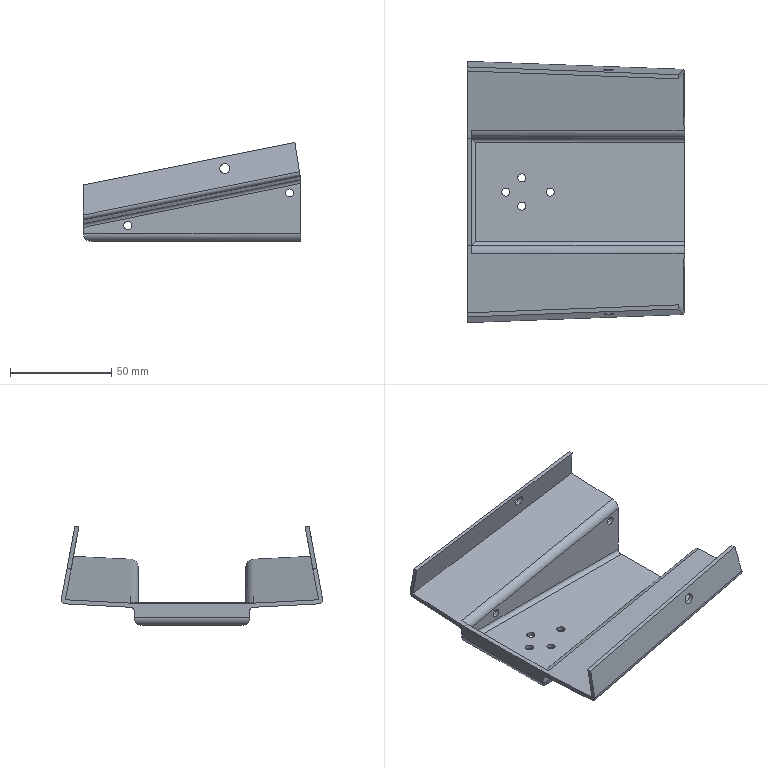Part | STEP file | 1-69.1 | 1 solid | 44 faces | box 107.541 x 129.236 x 49 mm | volume 41609 mm3 | cylinder 22 | plane 14 | spline 8 | commonest cylinder face diameters 4 x15 8 x5 5 x2